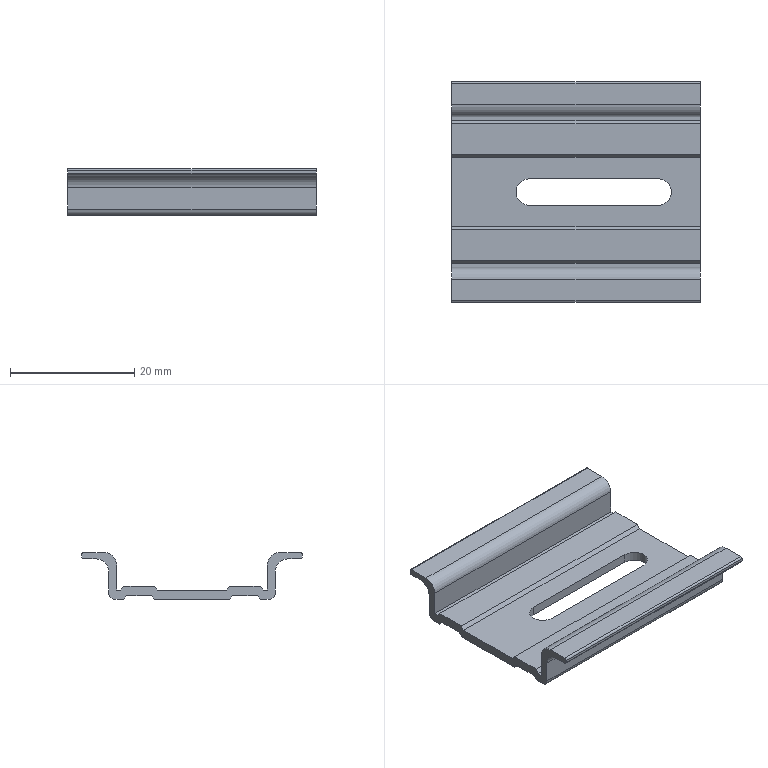Part | NX | features 5003_023_DRAL-5100-100 2 | 1 solid | 44 faces | box 40 x 35.457 x 7.5 mm | volume 2447 mm3 | plane 32 | cylinder 12 | commonest cylinder face diameters 0.6 x4 4 x4 2 x2 4.25 x2
STEP:
#1=CARTESIAN_POINT('',(243.525,-115.4,-99.5));
#2=VERTEX_POINT('',#1);
#3=CARTESIAN_POINT('',(243.525,-115.4,-103.));
#4=VERTEX_POINT('',#3);
#5=CARTESIAN_POINT('',(243.525,-115.4,-99.5));
#6=DIRECTION('',(0.,0.,-1.));
#7=VECTOR('',#6,1000.);
#8=LINE('',#5,#7);
#9=EDGE_CURVE('',#2,#4,#8,.T.);
#10=ORIENTED_EDGE('',*,*,#9,.T.);
#11=CARTESIAN_POINT('',(283.525,-115.4,-103.));
#12=VERTEX_POINT('',#11);
#13=CARTESIAN_POINT('',(283.525,-115.4,-103.));
#14=DIRECTION('',(-1.,0.,0.));
#15=VECTOR('',#14,1000.);
#16=LINE('',#13,#15);
#17=EDGE_CURVE('',#12,#4,#16,.T.);
#18=ORIENTED_EDGE('',*,*,#17,.F.);
#19=CARTESIAN_POINT('',(283.525,-115.4,-99.5));
#20=VERTEX_POINT('',#19);
#21=CARTESIAN_POINT('',(283.525,-115.4,-99.5));
#22=DIRECTION('',(0.,0.,-1.));
#23=VECTOR('',#22,1000.);
#24=LINE('',#21,#23);
#25=EDGE_CURVE('',#20,#12,#24,.T.);
#26=ORIENTED_EDGE('',*,*,#25,.F.);
#27=CARTESIAN_POINT('',(283.525,-115.4,-99.5));
#28=DIRECTION('',(-1.,0.,0.));
#29=VECTOR('',#28,1000.);
#30=LINE('',#27,#29);
#31=EDGE_CURVE('',#20,#2,#30,.T.);
#32=ORIENTED_EDGE('',*,*,#31,.T.);
#33=EDGE_LOOP('',(#10,#18,#26,#32));
#34=FACE_BOUND('',#33,.T.);
#35=CARTESIAN_POINT('',(283.525,-115.4,-99.5));
#36=DIRECTION('',(0.,1.,0.));
#37=DIRECTION('',(-1.,0.,0.));
#38=AXIS2_PLACEMENT_3D('',#35,#36,#37);
#39=PLANE('',#38);
#40=ADVANCED_FACE('',(#34),#39,.F.);
#41=CARTESIAN_POINT('',(243.525,-114.4,-104.));
#42=VERTEX_POINT('',#41);
#43=CARTESIAN_POINT('',(243.525,-114.4,-103.));
#44=DIRECTION('',(1.,0.,0.));
#45=DIRECTION('',(0.,1.,0.));
#46=AXIS2_PLACEMENT_3D('',#43,#44,#45);
#47=CIRCLE('',#46,1.);
#48=EDGE_CURVE('',#4,#42,#47,.T.);
#49=ORIENTED_EDGE('',*,*,#48,.T.);
#50=CARTESIAN_POINT('',(283.525,-114.4,-104.));
#51=VERTEX_POINT('',#50);
#52=CARTESIAN_POINT('',(283.525,-114.4,-104.));
#53=DIRECTION('',(-1.,0.,0.));
#54=VECTOR('',#53,1000.);
#55=LINE('',#52,#54);
#56=EDGE_CURVE('',#51,#42,#55,.T.);
#57=ORIENTED_EDGE('',*,*,#56,.F.);
#58=CARTESIAN_POINT('',(283.525,-114.4,-103.));
#59=DIRECTION('',(1.,0.,0.));
#60=DIRECTION('',(0.,1.,0.));
#61=AXIS2_PLACEMENT_3D('',#58,#59,#60);
#62=CIRCLE('',#61,1.);
#63=EDGE_CURVE('',#12,#51,#62,.T.);
#64=ORIENTED_EDGE('',*,*,#63,.F.);
#65=ORIENTED_EDGE('',*,*,#17,.T.);
#66=EDGE_LOOP('',(#49,#57,#64,#65));
#67=FACE_BOUND('',#66,.T.);
#68=CARTESIAN_POINT('',(283.525,-114.4,-103.));
#69=DIRECTION('',(-1.,0.,0.));
#70=DIRECTION('',(0.,-1.,0.));
#71=AXIS2_PLACEMENT_3D('',#68,#69,#70);
#72=CYLINDRICAL_SURFACE('',#71,1.);
#73=ADVANCED_FACE('',(#67),#72,.T.);
#74=CARTESIAN_POINT('',(243.525,-113.,-104.));
#75=VERTEX_POINT('',#74);
#76=CARTESIAN_POINT('',(243.525,-113.,-104.));
#77=DIRECTION('',(0.,-1.,0.));
#78=VECTOR('',#77,1000.);
#79=LINE('',#76,#78);
#80=EDGE_CURVE('',#75,#42,#79,.T.);
#81=ORIENTED_EDGE('',*,*,#80,.F.);
#82=CARTESIAN_POINT('',(283.525,-113.,-104.));
#83=VERTEX_POINT('',#82);
#84=CARTESIAN_POINT('',(283.525,-113.,-104.));
#85=DIRECTION('',(-1.,0.,0.));
#86=VECTOR('',#85,1000.);
#87=LINE('',#84,#86);
#88=EDGE_CURVE('',#83,#75,#87,.T.);
#89=ORIENTED_EDGE('',*,*,#88,.F.);
#90=CARTESIAN_POINT('',(283.525,-113.,-104.));
#91=DIRECTION('',(0.,-1.,0.));
#92=VECTOR('',#91,1000.);
#93=LINE('',#90,#92);
#94=EDGE_CURVE('',#83,#51,#93,.T.);
#95=ORIENTED_EDGE('',*,*,#94,.T.);
#96=ORIENTED_EDGE('',*,*,#56,.T.);
#97=EDGE_LOOP('',(#81,#89,#95,#96));
#98=FACE_BOUND('',#97,.T.);
#99=CARTESIAN_POINT('',(283.525,-113.,-104.));
#100=DIRECTION('',(0.,0.,-1.));
#101=DIRECTION('',(0.,1.,0.));
#102=AXIS2_PLACEMENT_3D('',#99,#100,#101);
#103=PLANE('',#102);
#104=ADVANCED_FACE('',(#98),#103,.T.);
#105=CARTESIAN_POINT('',(243.525,-112.5,-103.4));
#106=VERTEX_POINT('',#105);
#107=CARTESIAN_POINT('',(243.525,-112.5,-103.4));
#108=DIRECTION('',(0.,-0.6402,-0.7682));
#109=VECTOR('',#108,1000.);
#110=LINE('',#107,#109);
#111=EDGE_CURVE('',#106,#75,#110,.T.);
#112=ORIENTED_EDGE('',*,*,#111,.F.);
#113=CARTESIAN_POINT('',(283.525,-112.5,-103.4));
#114=VERTEX_POINT('',#113);
#115=CARTESIAN_POINT('',(283.525,-112.5,-103.4));
#116=DIRECTION('',(-1.,0.,0.));
#117=VECTOR('',#116,1000.);
#118=LINE('',#115,#117);
#119=EDGE_CURVE('',#114,#106,#118,.T.);
#120=ORIENTED_EDGE('',*,*,#119,.F.);
#121=CARTESIAN_POINT('',(283.525,-112.5,-103.4));
#122=DIRECTION('',(0.,-0.6402,-0.7682));
#123=VECTOR('',#122,1000.);
#124=LINE('',#121,#123);
#125=EDGE_CURVE('',#114,#83,#124,.T.);
#126=ORIENTED_EDGE('',*,*,#125,.T.);
#127=ORIENTED_EDGE('',*,*,#88,.T.);
#128=EDGE_LOOP('',(#112,#120,#126,#127));
#129=FACE_BOUND('',#128,.T.);
#130=CARTESIAN_POINT('',(283.525,-112.5,-103.4));
#131=DIRECTION('',(0.,0.7682,-0.6402));
#132=DIRECTION('',(0.,0.6402,0.7682));
#133=AXIS2_PLACEMENT_3D('',#130,#131,#132);
#134=PLANE('',#133);
#135=ADVANCED_FACE('',(#129),#134,.T.);
#136=CARTESIAN_POINT('',(243.525,-108.5,-103.4));
#137=VERTEX_POINT('',#136);
#138=CARTESIAN_POINT('',(243.525,-108.5,-103.4));
#139=DIRECTION('',(0.,-1.,0.));
#140=VECTOR('',#139,1000.);
#141=LINE('',#138,#140);
#142=EDGE_CURVE('',#137,#106,#141,.T.);
#143=ORIENTED_EDGE('',*,*,#142,.F.);
#144=CARTESIAN_POINT('',(283.525,-108.5,-103.4));
#145=VERTEX_POINT('',#144);
#146=CARTESIAN_POINT('',(283.525,-108.5,-103.4));
#147=DIRECTION('',(-1.,0.,0.));
#148=VECTOR('',#147,1000.);
#149=LINE('',#146,#148);
#150=EDGE_CURVE('',#145,#137,#149,.T.);
#151=ORIENTED_EDGE('',*,*,#150,.F.);
#152=CARTESIAN_POINT('',(283.525,-108.5,-103.4));
#153=DIRECTION('',(0.,-1.,0.));
#154=VECTOR('',#153,1000.);
#155=LINE('',#152,#154);
#156=EDGE_CURVE('',#145,#114,#155,.T.);
#157=ORIENTED_EDGE('',*,*,#156,.T.);
#158=ORIENTED_EDGE('',*,*,#119,.T.);
#159=EDGE_LOOP('',(#143,#151,#157,#158));
#160=FACE_BOUND('',#159,.T.);
#161=CARTESIAN_POINT('',(283.525,-108.5,-103.4));
#162=DIRECTION('',(0.,0.,-1.));
#163=DIRECTION('',(0.,1.,0.));
#164=AXIS2_PLACEMENT_3D('',#161,#162,#163);
#165=PLANE('',#164);
#166=ADVANCED_FACE('',(#160),#165,.T.);
#167=CARTESIAN_POINT('',(243.525,-108.,-104.));
#168=VERTEX_POINT('',#167);
#169=CARTESIAN_POINT('',(243.525,-108.,-104.));
#170=DIRECTION('',(0.,-0.6402,0.7682));
#171=VECTOR('',#170,1000.);
#172=LINE('',#169,#171);
#173=EDGE_CURVE('',#168,#137,#172,.T.);
#174=ORIENTED_EDGE('',*,*,#173,.F.);
#175=CARTESIAN_POINT('',(283.525,-108.,-104.));
#176=VERTEX_POINT('',#175);
#177=CARTESIAN_POINT('',(283.525,-108.,-104.));
#178=DIRECTION('',(-1.,0.,0.));
#179=VECTOR('',#178,1000.);
#180=LINE('',#177,#179);
#181=EDGE_CURVE('',#176,#168,#180,.T.);
#182=ORIENTED_EDGE('',*,*,#181,.F.);
#183=CARTESIAN_POINT('',(283.525,-108.,-104.));
#184=DIRECTION('',(0.,-0.6402,0.7682));
#185=VECTOR('',#184,1000.);
#186=LINE('',#183,#185);
#187=EDGE_CURVE('',#176,#145,#186,.T.);
#188=ORIENTED_EDGE('',*,*,#187,.T.);
#189=ORIENTED_EDGE('',*,*,#150,.T.);
#190=EDGE_LOOP('',(#174,#182,#188,#189));
#191=FACE_BOUND('',#190,.T.);
#192=CARTESIAN_POINT('',(283.525,-108.,-104.));
#193=DIRECTION('',(0.,-0.7682,-0.6402));
#194=DIRECTION('',(0.,0.6402,-0.7682));
#195=AXIS2_PLACEMENT_3D('',#192,#193,#194);
#196=PLANE('',#195);
#197=ADVANCED_FACE('',(#191),#196,.T.);
#198=CARTESIAN_POINT('',(256.005,-104.125,-104.));
#199=VERTEX_POINT('',#198);
#200=CARTESIAN_POINT('',(256.005,-99.875,-104.));
#201=VERTEX_POINT('',#200);
#202=CARTESIAN_POINT('',(256.005,-102.,-104.));
#203=DIRECTION('',(0.,0.,-1.));
#204=DIRECTION('',(0.,1.,0.));
#205=AXIS2_PLACEMENT_3D('',#202,#203,#204);
#206=CIRCLE('',#205,2.125);
#207=EDGE_CURVE('',#199,#201,#206,.T.);
#208=ORIENTED_EDGE('',*,*,#207,.F.);
#209=CARTESIAN_POINT('',(276.755,-104.125,-104.));
#210=VERTEX_POINT('',#209);
#211=CARTESIAN_POINT('',(283.525,-104.125,-104.));
#212=DIRECTION('',(-1.,0.,0.));
#213=VECTOR('',#212,1000.);
#214=LINE('',#211,#213);
#215=EDGE_CURVE('',#210,#199,#214,.T.);
#216=ORIENTED_EDGE('',*,*,#215,.F.);
#217=CARTESIAN_POINT('',(276.755,-99.875,-104.));
#218=VERTEX_POINT('',#217);
#219=CARTESIAN_POINT('',(276.755,-102.,-104.));
#220=DIRECTION('',(0.,0.,-1.));
#221=DIRECTION('',(0.,1.,0.));
#222=AXIS2_PLACEMENT_3D('',#219,#220,#221);
#223=CIRCLE('',#222,2.125);
#224=EDGE_CURVE('',#218,#210,#223,.T.);
#225=ORIENTED_EDGE('',*,*,#224,.F.);
#226=CARTESIAN_POINT('',(283.525,-99.875,-104.));
#227=DIRECTION('',(-1.,0.,0.));
#228=VECTOR('',#227,1000.);
#229=LINE('',#226,#228);
#230=EDGE_CURVE('',#218,#201,#229,.T.);
#231=ORIENTED_EDGE('',*,*,#230,.T.);
#232=EDGE_LOOP('',(#208,#216,#225,#231));
#233=FACE_BOUND('',#232,.T.);
#234=CARTESIAN_POINT('',(243.525,-96.,-104.));
#235=VERTEX_POINT('',#234);
#236=CARTESIAN_POINT('',(243.525,-96.,-104.));
#237=DIRECTION('',(0.,-1.,0.));
#238=VECTOR('',#237,1000.);
#239=LINE('',#236,#238);
#240=EDGE_CURVE('',#235,#168,#239,.T.);
#241=ORIENTED_EDGE('',*,*,#240,.F.);
#242=CARTESIAN_POINT('',(283.525,-96.,-104.));
#243=VERTEX_POINT('',#242);
#244=CARTESIAN_POINT('',(283.525,-96.,-104.));
#245=DIRECTION('',(-1.,0.,0.));
#246=VECTOR('',#245,1000.);
#247=LINE('',#244,#246);
#248=EDGE_CURVE('',#243,#235,#247,.T.);
#249=ORIENTED_EDGE('',*,*,#248,.F.);
#250=CARTESIAN_POINT('',(283.525,-96.,-104.));
#251=DIRECTION('',(0.,-1.,0.));
#252=VECTOR('',#251,1000.);
#253=LINE('',#250,#252);
#254=EDGE_CURVE('',#243,#176,#253,.T.);
#255=ORIENTED_EDGE('',*,*,#254,.T.);
#256=ORIENTED_EDGE('',*,*,#181,.T.);
#257=EDGE_LOOP('',(#241,#249,#255,#256));
#258=FACE_BOUND('',#257,.T.);
#259=CARTESIAN_POINT('',(283.525,-96.,-104.));
#260=DIRECTION('',(0.,0.,-1.));
#261=DIRECTION('',(0.,1.,0.));
#262=AXIS2_PLACEMENT_3D('',#259,#260,#261);
#263=PLANE('',#262);
#264=ADVANCED_FACE('',(#233,#258),#263,.T.);
#265=CARTESIAN_POINT('',(243.525,-95.5,-103.4));
#266=VERTEX_POINT('',#265);
#267=CARTESIAN_POINT('',(243.525,-96.,-104.));
#268=DIRECTION('',(0.,0.6402,0.7682));
#269=VECTOR('',#268,1000.);
#270=LINE('',#267,#269);
#271=EDGE_CURVE('',#235,#266,#270,.T.);
#272=ORIENTED_EDGE('',*,*,#271,.T.);
#273=CARTESIAN_POINT('',(283.525,-95.5,-103.4));
#274=VERTEX_POINT('',#273);
#275=CARTESIAN_POINT('',(283.525,-95.5,-103.4));
#276=DIRECTION('',(-1.,0.,0.));
#277=VECTOR('',#276,1000.);
#278=LINE('',#275,#277);
#279=EDGE_CURVE('',#274,#266,#278,.T.);
#280=ORIENTED_EDGE('',*,*,#279,.F.);
#281=CARTESIAN_POINT('',(283.525,-96.,-104.));
#282=DIRECTION('',(0.,0.6402,0.7682));
#283=VECTOR('',#282,1000.);
#284=LINE('',#281,#283);
#285=EDGE_CURVE('',#243,#274,#284,.T.);
#286=ORIENTED_EDGE('',*,*,#285,.F.);
#287=ORIENTED_EDGE('',*,*,#248,.T.);
#288=EDGE_LOOP('',(#272,#280,#286,#287));
#289=FACE_BOUND('',#288,.T.);
#290=CARTESIAN_POINT('',(283.525,-96.,-104.));
#291=DIRECTION('',(0.,-0.7682,0.6402));
#292=DIRECTION('',(0.,-0.6402,-0.7682));
#293=AXIS2_PLACEMENT_3D('',#290,#291,#292);
#294=PLANE('',#293);
#295=ADVANCED_FACE('',(#289),#294,.F.);
#296=CARTESIAN_POINT('',(243.525,-91.5,-103.4));
#297=VERTEX_POINT('',#296);
#298=CARTESIAN_POINT('',(243.525,-95.5,-103.4));
#299=DIRECTION('',(0.,1.,0.));
#300=VECTOR('',#299,1000.);
#301=LINE('',#298,#300);
#302=EDGE_CURVE('',#266,#297,#301,.T.);
#303=ORIENTED_EDGE('',*,*,#302,.T.);
#304=CARTESIAN_POINT('',(283.525,-91.5,-103.4));
#305=VERTEX_POINT('',#304);
#306=CARTESIAN_POINT('',(283.525,-91.5,-103.4));
#307=DIRECTION('',(-1.,0.,0.));
#308=VECTOR('',#307,1000.);
#309=LINE('',#306,#308);
#310=EDGE_CURVE('',#305,#297,#309,.T.);
#311=ORIENTED_EDGE('',*,*,#310,.F.);
#312=CARTESIAN_POINT('',(283.525,-95.5,-103.4));
#313=DIRECTION('',(0.,1.,0.));
#314=VECTOR('',#313,1000.);
#315=LINE('',#312,#314);
#316=EDGE_CURVE('',#274,#305,#315,.T.);
#317=ORIENTED_EDGE('',*,*,#316,.F.);
#318=ORIENTED_EDGE('',*,*,#279,.T.);
#319=EDGE_LOOP('',(#303,#311,#317,#318));
#320=FACE_BOUND('',#319,.T.);
#321=CARTESIAN_POINT('',(283.525,-95.5,-103.4));
#322=DIRECTION('',(0.,0.,1.));
#323=DIRECTION('',(0.,-1.,0.));
#324=AXIS2_PLACEMENT_3D('',#321,#322,#323);
#325=PLANE('',#324);
#326=ADVANCED_FACE('',(#320),#325,.F.);
#327=CARTESIAN_POINT('',(243.525,-91.,-104.));
#328=VERTEX_POINT('',#327);
#329=CARTESIAN_POINT('',(243.525,-91.5,-103.4));
#330=DIRECTION('',(0.,0.6402,-0.7682));
#331=VECTOR('',#330,1000.);
#332=LINE('',#329,#331);
#333=EDGE_CURVE('',#297,#328,#332,.T.);
#334=ORIENTED_EDGE('',*,*,#333,.T.);
#335=CARTESIAN_POINT('',(283.525,-91.,-104.));
#336=VERTEX_POINT('',#335);
#337=CARTESIAN_POINT('',(283.525,-91.,-104.));
#338=DIRECTION('',(-1.,0.,0.));
#339=VECTOR('',#338,1000.);
#340=LINE('',#337,#339);
#341=EDGE_CURVE('',#336,#328,#340,.T.);
#342=ORIENTED_EDGE('',*,*,#341,.F.);
#343=CARTESIAN_POINT('',(283.525,-91.5,-103.4));
#344=DIRECTION('',(0.,0.6402,-0.7682));
#345=VECTOR('',#344,1000.);
#346=LINE('',#343,#345);
#347=EDGE_CURVE('',#305,#336,#346,.T.);
#348=ORIENTED_EDGE('',*,*,#347,.F.);
#349=ORIENTED_EDGE('',*,*,#310,.T.);
#350=EDGE_LOOP('',(#334,#342,#348,#349));
#351=FACE_BOUND('',#350,.T.);
#352=CARTESIAN_POINT('',(283.525,-91.5,-103.4));
#353=DIRECTION('',(0.,0.7682,0.6402));
#354=DIRECTION('',(0.,-0.6402,0.7682));
#355=AXIS2_PLACEMENT_3D('',#352,#353,#354);
#356=PLANE('',#355);
#357=ADVANCED_FACE('',(#351),#356,.F.);
#358=CARTESIAN_POINT('',(243.525,-89.6,-104.));
#359=VERTEX_POINT('',#358);
#360=CARTESIAN_POINT('',(243.525,-91.,-104.));
#361=DIRECTION('',(0.,1.,0.));
#362=VECTOR('',#361,1000.);
#363=LINE('',#360,#362);
#364=EDGE_CURVE('',#328,#359,#363,.T.);
#365=ORIENTED_EDGE('',*,*,#364,.T.);
#366=CARTESIAN_POINT('',(283.525,-89.6,-104.));
#367=VERTEX_POINT('',#366);
#368=CARTESIAN_POINT('',(283.525,-89.6,-104.));
#369=DIRECTION('',(-1.,0.,0.));
#370=VECTOR('',#369,1000.);
#371=LINE('',#368,#370);
#372=EDGE_CURVE('',#367,#359,#371,.T.);
#373=ORIENTED_EDGE('',*,*,#372,.F.);
#374=CARTESIAN_POINT('',(283.525,-91.,-104.));
#375=DIRECTION('',(0.,1.,0.));
#376=VECTOR('',#375,1000.);
#377=LINE('',#374,#376);
#378=EDGE_CURVE('',#336,#367,#377,.T.);
#379=ORIENTED_EDGE('',*,*,#378,.F.);
#380=ORIENTED_EDGE('',*,*,#341,.T.);
#381=EDGE_LOOP('',(#365,#373,#379,#380));
#382=FACE_BOUND('',#381,.T.);
#383=CARTESIAN_POINT('',(283.525,-91.,-104.));
#384=DIRECTION('',(0.,0.,1.));
#385=DIRECTION('',(0.,-1.,0.));
#386=AXIS2_PLACEMENT_3D('',#383,#384,#385);
#387=PLANE('',#386);
#388=ADVANCED_FACE('',(#382),#387,.F.);
#389=CARTESIAN_POINT('',(243.525,-88.6,-103.));
#390=VERTEX_POINT('',#389);
#391=CARTESIAN_POINT('',(243.525,-89.6,-103.));
#392=DIRECTION('',(-1.,0.,0.));
#393=DIRECTION('',(0.,-1.,0.));
#394=AXIS2_PLACEMENT_3D('',#391,#392,#393);
#395=CIRCLE('',#394,1.);
#396=EDGE_CURVE('',#390,#359,#395,.T.);
#397=ORIENTED_EDGE('',*,*,#396,.F.);
#398=CARTESIAN_POINT('',(283.525,-88.6,-103.));
#399=VERTEX_POINT('',#398);
#400=CARTESIAN_POINT('',(283.525,-88.6,-103.));
#401=DIRECTION('',(-1.,0.,0.));
#402=VECTOR('',#401,1000.);
#403=LINE('',#400,#402);
#404=EDGE_CURVE('',#399,#390,#403,.T.);
#405=ORIENTED_EDGE('',*,*,#404,.F.);
#406=CARTESIAN_POINT('',(283.525,-89.6,-103.));
#407=DIRECTION('',(-1.,0.,0.));
#408=DIRECTION('',(0.,-1.,0.));
#409=AXIS2_PLACEMENT_3D('',#406,#407,#408);
#410=CIRCLE('',#409,1.);
#411=EDGE_CURVE('',#399,#367,#410,.T.);
#412=ORIENTED_EDGE('',*,*,#411,.T.);
#413=ORIENTED_EDGE('',*,*,#372,.T.);
#414=EDGE_LOOP('',(#397,#405,#412,#413));
#415=FACE_BOUND('',#414,.T.);
#416=CARTESIAN_POINT('',(283.525,-89.6,-103.));
#417=DIRECTION('',(-1.,0.,0.));
#418=DIRECTION('',(0.,-1.,0.));
#419=AXIS2_PLACEMENT_3D('',#416,#417,#418);
#420=CYLINDRICAL_SURFACE('',#419,1.);
#421=ADVANCED_FACE('',(#415),#420,.T.);
#422=CARTESIAN_POINT('',(243.525,-88.6,-99.5));
#423=VERTEX_POINT('',#422);
#424=CARTESIAN_POINT('',(243.525,-88.6,-99.5));
#425=DIRECTION('',(0.,0.,-1.));
#426=VECTOR('',#425,1000.);
#427=LINE('',#424,#426);
#428=EDGE_CURVE('',#423,#390,#427,.T.);
#429=ORIENTED_EDGE('',*,*,#428,.F.);
#430=CARTESIAN_POINT('',(283.525,-88.6,-99.5));
#431=VERTEX_POINT('',#430);
#432=CARTESIAN_POINT('',(283.525,-88.6,-99.5));
#433=DIRECTION('',(-1.,0.,0.));
#434=VECTOR('',#433,1000.);
#435=LINE('',#432,#434);
#436=EDGE_CURVE('',#431,#423,#435,.T.);
#437=ORIENTED_EDGE('',*,*,#436,.F.);
#438=CARTESIAN_POINT('',(283.525,-88.6,-99.5));
#439=DIRECTION('',(0.,0.,-1.));
#440=VECTOR('',#439,1000.);
#441=LINE('',#438,#440);
#442=EDGE_CURVE('',#431,#399,#441,.T.);
#443=ORIENTED_EDGE('',*,*,#442,.T.);
#444=ORIENTED_EDGE('',*,*,#404,.T.);
#445=EDGE_LOOP('',(#429,#437,#443,#444));
#446=FACE_BOUND('',#445,.T.);
#447=CARTESIAN_POINT('',(283.525,-88.6,-99.5));
#448=DIRECTION('',(0.,1.,0.));
#449=DIRECTION('',(-1.,0.,0.));
#450=AXIS2_PLACEMENT_3D('',#447,#448,#449);
#451=PLANE('',#450);
#452=ADVANCED_FACE('',(#446),#451,.T.);
#453=CARTESIAN_POINT('',(243.525,-86.6,-97.5));
#454=VERTEX_POINT('',#453);
#455=CARTESIAN_POINT('',(243.525,-86.6,-99.5));
#456=DIRECTION('',(-1.,0.,0.));
#457=DIRECTION('',(0.,-1.,0.));
#458=AXIS2_PLACEMENT_3D('',#455,#456,#457);
#459=CIRCLE('',#458,2.);
#460=EDGE_CURVE('',#423,#454,#459,.T.);
#461=ORIENTED_EDGE('',*,*,#460,.T.);
#462=CARTESIAN_POINT('',(283.525,-86.6,-97.5));
#463=VERTEX_POINT('',#462);
#464=CARTESIAN_POINT('',(283.525,-86.6,-97.5));
#465=DIRECTION('',(-1.,0.,0.));
#466=VECTOR('',#465,1000.);
#467=LINE('',#464,#466);
#468=EDGE_CURVE('',#463,#454,#467,.T.);
#469=ORIENTED_EDGE('',*,*,#468,.F.);
#470=CARTESIAN_POINT('',(283.525,-86.6,-99.5));
#471=DIRECTION('',(-1.,0.,0.));
#472=DIRECTION('',(0.,-1.,0.));
#473=AXIS2_PLACEMENT_3D('',#470,#471,#472);
#474=CIRCLE('',#473,2.);
#475=EDGE_CURVE('',#431,#463,#474,.T.);
#476=ORIENTED_EDGE('',*,*,#475,.F.);
#477=ORIENTED_EDGE('',*,*,#436,.T.);
#478=EDGE_LOOP('',(#461,#469,#476,#477));
#479=FACE_BOUND('',#478,.T.);
#480=CARTESIAN_POINT('',(283.525,-86.6,-99.5));
#481=DIRECTION('',(-1.,0.,0.));
#482=DIRECTION('',(0.,-1.,0.));
#483=AXIS2_PLACEMENT_3D('',#480,#481,#482);
#484=CYLINDRICAL_SURFACE('',#483,2.);
#485=ADVANCED_FACE('',(#479),#484,.F.);
#486=CARTESIAN_POINT('',(243.525,-84.572,-97.5));
#487=VERTEX_POINT('',#486);
#488=CARTESIAN_POINT('',(243.525,-86.6,-97.5));
#489=DIRECTION('',(0.,1.,0.));
#490=VECTOR('',#489,1000.);
#491=LINE('',#488,#490);
#492=EDGE_CURVE('',#454,#487,#491,.T.);
#493=ORIENTED_EDGE('',*,*,#492,.T.);
#494=CARTESIAN_POINT('',(283.525,-84.572,-97.5));
#495=VERTEX_POINT('',#494);
#496=CARTESIAN_POINT('',(283.525,-84.572,-97.5));
#497=DIRECTION('',(-1.,0.,0.));
#498=VECTOR('',#497,1000.);
#499=LINE('',#496,#498);
#500=EDGE_CURVE('',#495,#487,#499,.T.);
#501=ORIENTED_EDGE('',*,*,#500,.F.);
#502=CARTESIAN_POINT('',(283.525,-86.6,-97.5));
#503=DIRECTION('',(0.,1.,0.));
#504=VECTOR('',#503,1000.);
#505=LINE('',#502,#504);
#506=EDGE_CURVE('',#463,#495,#505,.T.);
#507=ORIENTED_EDGE('',*,*,#506,.F.);
#508=ORIENTED_EDGE('',*,*,#468,.T.);
#509=EDGE_LOOP('',(#493,#501,#507,#508));
#510=FACE_BOUND('',#509,.T.);
#511=CARTESIAN_POINT('',(283.525,-86.6,-97.5));
#512=DIRECTION('',(0.,0.,1.));
#513=DIRECTION('',(0.,-1.,0.));
#514=AXIS2_PLACEMENT_3D('',#511,#512,#513);
#515=PLANE('',#514);
#516=ADVANCED_FACE('',(#510),#515,.F.);
#517=CARTESIAN_POINT('',(243.525,-84.272,-97.2));
#518=VERTEX_POINT('',#517);
#519=CARTESIAN_POINT('',(243.525,-84.572,-97.2));
#520=DIRECTION('',(-1.,0.,0.));
#521=DIRECTION('',(0.,-1.,0.));
#522=AXIS2_PLACEMENT_3D('',#519,#520,#521);
#523=CIRCLE('',#522,0.3);
#524=EDGE_CURVE('',#518,#487,#523,.T.);
#525=ORIENTED_EDGE('',*,*,#524,.F.);
#526=CARTESIAN_POINT('',(283.525,-84.272,-97.2));
#527=VERTEX_POINT('',#526);
#528=CARTESIAN_POINT('',(283.525,-84.272,-97.2));
#529=DIRECTION('',(-1.,0.,0.));
#530=VECTOR('',#529,1000.);
#531=LINE('',#528,#530);
#532=EDGE_CURVE('',#527,#518,#531,.T.);
#533=ORIENTED_EDGE('',*,*,#532,.F.);
#534=CARTESIAN_POINT('',(283.525,-84.572,-97.2));
#535=DIRECTION('',(-1.,0.,0.));
#536=DIRECTION('',(0.,-1.,0.));
#537=AXIS2_PLACEMENT_3D('',#534,#535,#536);
#538=CIRCLE('',#537,0.3);
#539=EDGE_CURVE('',#527,#495,#538,.T.);
#540=ORIENTED_EDGE('',*,*,#539,.T.);
#541=ORIENTED_EDGE('',*,*,#500,.T.);
#542=EDGE_LOOP('',(#525,#533,#540,#541));
#543=FACE_BOUND('',#542,.T.);
#544=CARTESIAN_POINT('',(283.525,-84.572,-97.2));
#545=DIRECTION('',(-1.,0.,0.));
#546=DIRECTION('',(0.,-1.,0.));
#547=AXIS2_PLACEMENT_3D('',#544,#545,#546);
#548=CYLINDRICAL_SURFACE('',#547,0.3);
#549=ADVANCED_FACE('',(#543),#548,.T.);
#550=CARTESIAN_POINT('',(243.525,-84.272,-96.8));
#551=VERTEX_POINT('',#550);
#552=CARTESIAN_POINT('',(243.525,-84.272,-97.2));
#553=DIRECTION('',(0.,0.,1.));
#554=VECTOR('',#553,1000.);
#555=LINE('',#552,#554);
#556=EDGE_CURVE('',#518,#551,#555,.T.);
#557=ORIENTED_EDGE('',*,*,#556,.T.);
#558=CARTESIAN_POINT('',(283.525,-84.272,-96.8));
#559=VERTEX_POINT('',#558);
#560=CARTESIAN_POINT('',(283.525,-84.272,-96.8));
#561=DIRECTION('',(-1.,0.,0.));
#562=VECTOR('',#561,1000.);
#563=LINE('',#560,#562);
#564=EDGE_CURVE('',#559,#551,#563,.T.);
#565=ORIENTED_EDGE('',*,*,#564,.F.);
#566=CARTESIAN_POINT('',(283.525,-84.272,-97.2));
#567=DIRECTION('',(0.,0.,1.));
#568=VECTOR('',#567,1000.);
#569=LINE('',#566,#568);
#570=EDGE_CURVE('',#527,#559,#569,.T.);
#571=ORIENTED_EDGE('',*,*,#570,.F.);
#572=ORIENTED_EDGE('',*,*,#532,.T.);
#573=EDGE_LOOP('',(#557,#565,#571,#572));
#574=FACE_BOUND('',#573,.T.);
#575=CARTESIAN_POINT('',(283.525,-84.272,-97.2));
#576=DIRECTION('',(0.,-1.,0.));
#577=DIRECTION('',(1.,0.,0.));
#578=AXIS2_PLACEMENT_3D('',#575,#576,#577);
#579=PLANE('',#578);
#580=ADVANCED_FACE('',(#574),#579,.F.);
#581=CARTESIAN_POINT('',(243.525,-84.572,-96.5));
#582=VERTEX_POINT('',#581);
#583=CARTESIAN_POINT('',(243.525,-84.572,-96.8));
#584=DIRECTION('',(-1.,0.,0.));
#585=DIRECTION('',(0.,-1.,0.));
#586=AXIS2_PLACEMENT_3D('',#583,#584,#585);
#587=CIRCLE('',#586,0.3);
#588=EDGE_CURVE('',#582,#551,#587,.T.);
#589=ORIENTED_EDGE('',*,*,#588,.F.);
#590=CARTESIAN_POINT('',(283.525,-84.572,-96.5));
#591=VERTEX_POINT('',#590);
#592=CARTESIAN_POINT('',(283.525,-84.572,-96.5));
#593=DIRECTION('',(-1.,0.,0.));
#594=VECTOR('',#593,1000.);
#595=LINE('',#592,#594);
#596=EDGE_CURVE('',#591,#582,#595,.T.);
#597=ORIENTED_EDGE('',*,*,#596,.F.);
#598=CARTESIAN_POINT('',(283.525,-84.572,-96.8));
#599=DIRECTION('',(-1.,0.,0.));
#600=DIRECTION('',(0.,-1.,0.));
#601=AXIS2_PLACEMENT_3D('',#598,#599,#600);
#602=CIRCLE('',#601,0.3);
#603=EDGE_CURVE('',#591,#559,#602,.T.);
#604=ORIENTED_EDGE('',*,*,#603,.T.);
#605=ORIENTED_EDGE('',*,*,#564,.T.);
#606=EDGE_LOOP('',(#589,#597,#604,#605));
#607=FACE_BOUND('',#606,.T.);
#608=CARTESIAN_POINT('',(283.525,-84.572,-96.8));
#609=DIRECTION('',(-1.,0.,0.));
#610=DIRECTION('',(0.,-1.,0.));
#611=AXIS2_PLACEMENT_3D('',#608,#609,#610);
#612=CYLINDRICAL_SURFACE('',#611,0.3);
#613=ADVANCED_FACE('',(#607),#612,.T.);
#614=CARTESIAN_POINT('',(243.525,-87.9,-96.5));
#615=VERTEX_POINT('',#614);
#616=CARTESIAN_POINT('',(243.525,-84.572,-96.5));
#617=DIRECTION('',(0.,-1.,0.));
#618=VECTOR('',#617,1000.);
#619=LINE('',#616,#618);
#620=EDGE_CURVE('',#582,#615,#619,.T.);
#621=ORIENTED_EDGE('',*,*,#620,.T.);
#622=CARTESIAN_POINT('',(283.525,-87.9,-96.5));
#623=VERTEX_POINT('',#622);
#624=CARTESIAN_POINT('',(283.525,-87.9,-96.5));
#625=DIRECTION('',(-1.,0.,0.));
#626=VECTOR('',#625,1000.);
#627=LINE('',#624,#626);
#628=EDGE_CURVE('',#623,#615,#627,.T.);
#629=ORIENTED_EDGE('',*,*,#628,.F.);
#630=CARTESIAN_POINT('',(283.525,-84.572,-96.5));
#631=DIRECTION('',(0.,-1.,0.));
#632=VECTOR('',#631,1000.);
#633=LINE('',#630,#632);
#634=EDGE_CURVE('',#591,#623,#633,.T.);
#635=ORIENTED_EDGE('',*,*,#634,.F.);
#636=ORIENTED_EDGE('',*,*,#596,.T.);
#637=EDGE_LOOP('',(#621,#629,#635,#636));
#638=FACE_BOUND('',#637,.T.);
#639=CARTESIAN_POINT('',(283.525,-84.572,-96.5));
#640=DIRECTION('',(0.,0.,-1.));
#641=DIRECTION('',(0.,1.,0.));
#642=AXIS2_PLACEMENT_3D('',#639,#640,#641);
#643=PLANE('',#642);
#644=ADVANCED_FACE('',(#638),#643,.F.);
#645=CARTESIAN_POINT('',(243.525,-89.9,-98.5));
#646=VERTEX_POINT('',#645);
#647=CARTESIAN_POINT('',(243.525,-87.9,-98.5));
#648=DIRECTION('',(-1.,0.,0.));
#649=DIRECTION('',(0.,-1.,0.));
#650=AXIS2_PLACEMENT_3D('',#647,#648,#649);
#651=CIRCLE('',#650,2.);
#652=EDGE_CURVE('',#646,#615,#651,.T.);
#653=ORIENTED_EDGE('',*,*,#652,.F.);
#654=CARTESIAN_POINT('',(283.525,-89.9,-98.5));
#655=VERTEX_POINT('',#654);
#656=CARTESIAN_POINT('',(283.525,-89.9,-98.5));
#657=DIRECTION('',(-1.,0.,0.));
#658=VECTOR('',#657,1000.);
#659=LINE('',#656,#658);
#660=EDGE_CURVE('',#655,#646,#659,.T.);
#661=ORIENTED_EDGE('',*,*,#660,.F.);
#662=CARTESIAN_POINT('',(283.525,-87.9,-98.5));
#663=DIRECTION('',(-1.,0.,0.));
#664=DIRECTION('',(0.,-1.,0.));
#665=AXIS2_PLACEMENT_3D('',#662,#663,#664);
#666=CIRCLE('',#665,2.);
#667=EDGE_CURVE('',#655,#623,#666,.T.);
#668=ORIENTED_EDGE('',*,*,#667,.T.);
#669=ORIENTED_EDGE('',*,*,#628,.T.);
#670=EDGE_LOOP('',(#653,#661,#668,#669));
#671=FACE_BOUND('',#670,.T.);
#672=CARTESIAN_POINT('',(283.525,-87.9,-98.5));
#673=DIRECTION('',(-1.,0.,0.));
#674=DIRECTION('',(0.,-1.,0.));
#675=AXIS2_PLACEMENT_3D('',#672,#673,#674);
#676=CYLINDRICAL_SURFACE('',#675,2.);
#677=ADVANCED_FACE('',(#671),#676,.T.);
#678=CARTESIAN_POINT('',(243.525,-89.9,-102.5));
#679=VERTEX_POINT('',#678);
#680=CARTESIAN_POINT('',(243.525,-89.9,-98.5));
#681=DIRECTION('',(0.,0.,-1.));
#682=VECTOR('',#681,1000.);
#683=LINE('',#680,#682);
#684=EDGE_CURVE('',#646,#679,#683,.T.);
#685=ORIENTED_EDGE('',*,*,#684,.T.);
#686=CARTESIAN_POINT('',(283.525,-89.9,-102.5));
#687=VERTEX_POINT('',#686);
#688=CARTESIAN_POINT('',(283.525,-89.9,-102.5));
#689=DIRECTION('',(-1.,0.,0.));
#690=VECTOR('',#689,1000.);
#691=LINE('',#688,#690);
#692=EDGE_CURVE('',#687,#679,#691,.T.);
#693=ORIENTED_EDGE('',*,*,#692,.F.);
#694=CARTESIAN_POINT('',(283.525,-89.9,-98.5));
#695=DIRECTION('',(0.,0.,-1.));
#696=VECTOR('',#695,1000.);
#697=LINE('',#694,#696);
#698=EDGE_CURVE('',#655,#687,#697,.T.);
#699=ORIENTED_EDGE('',*,*,#698,.F.);
#700=ORIENTED_EDGE('',*,*,#660,.T.);
#701=EDGE_LOOP('',(#685,#693,#699,#700));
#702=FACE_BOUND('',#701,.T.);
#703=CARTESIAN_POINT('',(283.525,-89.9,-98.5));
#704=DIRECTION('',(0.,1.,0.));
#705=DIRECTION('',(0.,0.,1.));
#706=AXIS2_PLACEMENT_3D('',#703,#704,#705);
#707=PLANE('',#706);
#708=ADVANCED_FACE('',(#702),#707,.F.);
#709=CARTESIAN_POINT('',(243.525,-90.558,-102.5));
#710=VERTEX_POINT('',#709);
#711=CARTESIAN_POINT('',(243.525,-89.9,-102.5));
#712=DIRECTION('',(0.,-1.,0.));
#713=VECTOR('',#712,1000.);
#714=LINE('',#711,#713);
#715=EDGE_CURVE('',#679,#710,#714,.T.);
#716=ORIENTED_EDGE('',*,*,#715,.T.);
#717=CARTESIAN_POINT('',(283.525,-90.558,-102.5));
#718=VERTEX_POINT('',#717);
#719=CARTESIAN_POINT('',(283.525,-90.558,-102.5));
#720=DIRECTION('',(-1.,0.,0.));
#721=VECTOR('',#720,1000.);
#722=LINE('',#719,#721);
#723=EDGE_CURVE('',#718,#710,#722,.T.);
#724=ORIENTED_EDGE('',*,*,#723,.F.);
#725=CARTESIAN_POINT('',(283.525,-89.9,-102.5));
#726=DIRECTION('',(0.,-1.,0.));
#727=VECTOR('',#726,1000.);
#728=LINE('',#725,#727);
#729=EDGE_CURVE('',#687,#718,#728,.T.);
#730=ORIENTED_EDGE('',*,*,#729,.F.);
#731=ORIENTED_EDGE('',*,*,#692,.T.);
#732=EDGE_LOOP('',(#716,#724,#730,#731));
#733=FACE_BOUND('',#732,.T.);
#734=CARTESIAN_POINT('',(283.525,-89.9,-102.5));
#735=DIRECTION('',(0.,0.,-1.));
#736=DIRECTION('',(0.,1.,0.));
#737=AXIS2_PLACEMENT_3D('',#734,#735,#736);
#738=PLANE('',#737);
#739=ADVANCED_FACE('',(#733),#738,.F.);
#740=CARTESIAN_POINT('',(243.525,-91.058,-101.9));
#741=VERTEX_POINT('',#740);
#742=CARTESIAN_POINT('',(243.525,-90.558,-102.5));
#743=DIRECTION('',(0.,-0.6402,0.7682));
#744=VECTOR('',#743,1000.);
#745=LINE('',#742,#744);
#746=EDGE_CURVE('',#710,#741,#745,.T.);
#747=ORIENTED_EDGE('',*,*,#746,.T.);
#748=CARTESIAN_POINT('',(283.525,-91.058,-101.9));
#749=VERTEX_POINT('',#748);
#750=CARTESIAN_POINT('',(283.525,-91.058,-101.9));
#751=DIRECTION('',(-1.,0.,0.));
#752=VECTOR('',#751,1000.);
#753=LINE('',#750,#752);
#754=EDGE_CURVE('',#749,#741,#753,.T.);
#755=ORIENTED_EDGE('',*,*,#754,.F.);
#756=CARTESIAN_POINT('',(283.525,-90.558,-102.5));
#757=DIRECTION('',(0.,-0.6402,0.7682));
#758=VECTOR('',#757,1000.);
#759=LINE('',#756,#758);
#760=EDGE_CURVE('',#718,#749,#759,.T.);
#761=ORIENTED_EDGE('',*,*,#760,.F.);
#762=ORIENTED_EDGE('',*,*,#723,.T.);
#763=EDGE_LOOP('',(#747,#755,#761,#762));
#764=FACE_BOUND('',#763,.T.);
#765=CARTESIAN_POINT('',(283.525,-90.558,-102.5));
#766=DIRECTION('',(0.,-0.7682,-0.6402));
#767=DIRECTION('',(0.,0.6402,-0.7682));
#768=AXIS2_PLACEMENT_3D('',#765,#766,#767);
#769=PLANE('',#768);
#770=ADVANCED_FACE('',(#764),#769,.F.);
#771=CARTESIAN_POINT('',(243.525,-95.942,-101.9));
#772=VERTEX_POINT('',#771);
#773=CARTESIAN_POINT('',(243.525,-91.058,-101.9));
#774=DIRECTION('',(0.,-1.,0.));
#775=VECTOR('',#774,1000.);
#776=LINE('',#773,#775);
#777=EDGE_CURVE('',#741,#772,#776,.T.);
#778=ORIENTED_EDGE('',*,*,#777,.T.);
#779=CARTESIAN_POINT('',(283.525,-95.942,-101.9));
#780=VERTEX_POINT('',#779);
#781=CARTESIAN_POINT('',(283.525,-95.942,-101.9));
#782=DIRECTION('',(-1.,0.,0.));
#783=VECTOR('',#782,1000.);
#784=LINE('',#781,#783);
#785=EDGE_CURVE('',#780,#772,#784,.T.);
#786=ORIENTED_EDGE('',*,*,#785,.F.);
#787=CARTESIAN_POINT('',(283.525,-91.058,-101.9));
#788=DIRECTION('',(0.,-1.,0.));
#789=VECTOR('',#788,1000.);
#790=LINE('',#787,#789);
#791=EDGE_CURVE('',#749,#780,#790,.T.);
#792=ORIENTED_EDGE('',*,*,#791,.F.);
#793=ORIENTED_EDGE('',*,*,#754,.T.);
#794=EDGE_LOOP('',(#778,#786,#792,#793));
#795=FACE_BOUND('',#794,.T.);
#796=CARTESIAN_POINT('',(283.525,-91.058,-101.9));
#797=DIRECTION('',(0.,0.,-1.));
#798=DIRECTION('',(0.,1.,0.));
#799=AXIS2_PLACEMENT_3D('',#796,#797,#798);
#800=PLANE('',#799);
#801=ADVANCED_FACE('',(#795),#800,.F.);
#802=CARTESIAN_POINT('',(243.525,-96.442,-102.5));
#803=VERTEX_POINT('',#802);
#804=CARTESIAN_POINT('',(243.525,-95.942,-101.9));
#805=DIRECTION('',(0.,-0.6402,-0.7682));
#806=VECTOR('',#805,1000.);
#807=LINE('',#804,#806);
#808=EDGE_CURVE('',#772,#803,#807,.T.);
#809=ORIENTED_EDGE('',*,*,#808,.T.);
#810=CARTESIAN_POINT('',(283.525,-96.442,-102.5));
#811=VERTEX_POINT('',#810);
#812=CARTESIAN_POINT('',(283.525,-96.442,-102.5));
#813=DIRECTION('',(-1.,0.,0.));
#814=VECTOR('',#813,1000.);
#815=LINE('',#812,#814);
#816=EDGE_CURVE('',#811,#803,#815,.T.);
#817=ORIENTED_EDGE('',*,*,#816,.F.);
#818=CARTESIAN_POINT('',(283.525,-95.942,-101.9));
#819=DIRECTION('',(0.,-0.6402,-0.7682));
#820=VECTOR('',#819,1000.);
#821=LINE('',#818,#820);
#822=EDGE_CURVE('',#780,#811,#821,.T.);
#823=ORIENTED_EDGE('',*,*,#822,.F.);
#824=ORIENTED_EDGE('',*,*,#785,.T.);
#825=EDGE_LOOP('',(#809,#817,#823,#824));
#826=FACE_BOUND('',#825,.T.);
#827=CARTESIAN_POINT('',(283.525,-95.942,-101.9));
#828=DIRECTION('',(0.,0.7682,-0.6402));
#829=DIRECTION('',(0.,0.6402,0.7682));
#830=AXIS2_PLACEMENT_3D('',#827,#828,#829);
#831=PLANE('',#830);
#832=ADVANCED_FACE('',(#826),#831,.F.);
#833=CARTESIAN_POINT('',(256.005,-99.875,-102.5));
#834=VERTEX_POINT('',#833);
#835=CARTESIAN_POINT('',(256.005,-104.125,-102.5));
#836=VERTEX_POINT('',#835);
#837=CARTESIAN_POINT('',(256.005,-102.,-102.5));
#838=DIRECTION('',(0.,0.,1.));
#839=DIRECTION('',(0.,-1.,0.));
#840=AXIS2_PLACEMENT_3D('',#837,#838,#839);
#841=CIRCLE('',#840,2.125);
#842=EDGE_CURVE('',#834,#836,#841,.T.);
#843=ORIENTED_EDGE('',*,*,#842,.F.);
#844=CARTESIAN_POINT('',(276.755,-99.875,-102.5));
#845=VERTEX_POINT('',#844);
#846=CARTESIAN_POINT('',(256.005,-99.875,-102.5));
#847=DIRECTION('',(1.,0.,0.));
#848=VECTOR('',#847,1000.);
#849=LINE('',#846,#848);
#850=EDGE_CURVE('',#834,#845,#849,.T.);
#851=ORIENTED_EDGE('',*,*,#850,.T.);
#852=CARTESIAN_POINT('',(276.755,-104.125,-102.5));
#853=VERTEX_POINT('',#852);
#854=CARTESIAN_POINT('',(276.755,-102.,-102.5));
#855=DIRECTION('',(0.,0.,1.));
#856=DIRECTION('',(0.,-1.,0.));
#857=AXIS2_PLACEMENT_3D('',#854,#855,#856);
#858=CIRCLE('',#857,2.125);
#859=EDGE_CURVE('',#853,#845,#858,.T.);
#860=ORIENTED_EDGE('',*,*,#859,.F.);
#861=CARTESIAN_POINT('',(256.005,-104.125,-102.5));
#862=DIRECTION('',(1.,0.,0.));
#863=VECTOR('',#862,1000.);
#864=LINE('',#861,#863);
#865=EDGE_CURVE('',#836,#853,#864,.T.);
#866=ORIENTED_EDGE('',*,*,#865,.F.);
#867=EDGE_LOOP('',(#843,#851,#860,#866));
#868=FACE_BOUND('',#867,.T.);
#869=CARTESIAN_POINT('',(243.525,-107.558,-102.5));
#870=VERTEX_POINT('',#869);
#871=CARTESIAN_POINT('',(243.525,-107.558,-102.5));
#872=DIRECTION('',(0.,1.,0.));
#873=VECTOR('',#872,1000.);
#874=LINE('',#871,#873);
#875=EDGE_CURVE('',#870,#803,#874,.T.);
#876=ORIENTED_EDGE('',*,*,#875,.F.);
#877=CARTESIAN_POINT('',(283.525,-107.558,-102.5));
#878=VERTEX_POINT('',#877);
#879=CARTESIAN_POINT('',(283.525,-107.558,-102.5));
#880=DIRECTION('',(-1.,0.,0.));
#881=VECTOR('',#880,1000.);
#882=LINE('',#879,#881);
#883=EDGE_CURVE('',#878,#870,#882,.T.);
#884=ORIENTED_EDGE('',*,*,#883,.F.);
#885=CARTESIAN_POINT('',(283.525,-107.558,-102.5));
#886=DIRECTION('',(0.,1.,0.));
#887=VECTOR('',#886,1000.);
#888=LINE('',#885,#887);
#889=EDGE_CURVE('',#878,#811,#888,.T.);
#890=ORIENTED_EDGE('',*,*,#889,.T.);
#891=ORIENTED_EDGE('',*,*,#816,.T.);
#892=EDGE_LOOP('',(#876,#884,#890,#891));
#893=FACE_BOUND('',#892,.T.);
#894=CARTESIAN_POINT('',(283.525,-107.558,-102.5));
#895=DIRECTION('',(0.,0.,1.));
#896=DIRECTION('',(0.,-1.,0.));
#897=AXIS2_PLACEMENT_3D('',#894,#895,#896);
#898=PLANE('',#897);
#899=ADVANCED_FACE('',(#868,#893),#898,.T.);
#900=CARTESIAN_POINT('',(243.525,-108.058,-101.9));
#901=VERTEX_POINT('',#900);
#902=CARTESIAN_POINT('',(243.525,-108.058,-101.9));
#903=DIRECTION('',(0.,0.6402,-0.7682));
#904=VECTOR('',#903,1000.);
#905=LINE('',#902,#904);
#906=EDGE_CURVE('',#901,#870,#905,.T.);
#907=ORIENTED_EDGE('',*,*,#906,.F.);
#908=CARTESIAN_POINT('',(283.525,-108.058,-101.9));
#909=VERTEX_POINT('',#908);
#910=CARTESIAN_POINT('',(283.525,-108.058,-101.9));
#911=DIRECTION('',(-1.,0.,0.));
#912=VECTOR('',#911,1000.);
#913=LINE('',#910,#912);
#914=EDGE_CURVE('',#909,#901,#913,.T.);
#915=ORIENTED_EDGE('',*,*,#914,.F.);
#916=CARTESIAN_POINT('',(283.525,-108.058,-101.9));
#917=DIRECTION('',(0.,0.6402,-0.7682));
#918=VECTOR('',#917,1000.);
#919=LINE('',#916,#918);
#920=EDGE_CURVE('',#909,#878,#919,.T.);
#921=ORIENTED_EDGE('',*,*,#920,.T.);
#922=ORIENTED_EDGE('',*,*,#883,.T.);
#923=EDGE_LOOP('',(#907,#915,#921,#922));
#924=FACE_BOUND('',#923,.T.);
#925=CARTESIAN_POINT('',(283.525,-108.058,-101.9));
#926=DIRECTION('',(0.,0.7682,0.6402));
#927=DIRECTION('',(0.,-0.6402,0.7682));
#928=AXIS2_PLACEMENT_3D('',#925,#926,#927);
#929=PLANE('',#928);
#930=ADVANCED_FACE('',(#924),#929,.T.);
#931=CARTESIAN_POINT('',(243.525,-112.942,-101.9));
#932=VERTEX_POINT('',#931);
#933=CARTESIAN_POINT('',(243.525,-112.942,-101.9));
#934=DIRECTION('',(0.,1.,0.));
#935=VECTOR('',#934,1000.);
#936=LINE('',#933,#935);
#937=EDGE_CURVE('',#932,#901,#936,.T.);
#938=ORIENTED_EDGE('',*,*,#937,.F.);
#939=CARTESIAN_POINT('',(283.525,-112.942,-101.9));
#940=VERTEX_POINT('',#939);
#941=CARTESIAN_POINT('',(283.525,-112.942,-101.9));
#942=DIRECTION('',(-1.,0.,0.));
#943=VECTOR('',#942,1000.);
#944=LINE('',#941,#943);
#945=EDGE_CURVE('',#940,#932,#944,.T.);
#946=ORIENTED_EDGE('',*,*,#945,.F.);
#947=CARTESIAN_POINT('',(283.525,-112.942,-101.9));
#948=DIRECTION('',(0.,1.,0.));
#949=VECTOR('',#948,1000.);
#950=LINE('',#947,#949);
#951=EDGE_CURVE('',#940,#909,#950,.T.);
#952=ORIENTED_EDGE('',*,*,#951,.T.);
#953=ORIENTED_EDGE('',*,*,#914,.T.);
#954=EDGE_LOOP('',(#938,#946,#952,#953));
#955=FACE_BOUND('',#954,.T.);
#956=CARTESIAN_POINT('',(283.525,-112.942,-101.9));
#957=DIRECTION('',(0.,0.,1.));
#958=DIRECTION('',(0.,-1.,0.));
#959=AXIS2_PLACEMENT_3D('',#956,#957,#958);
#960=PLANE('',#959);
#961=ADVANCED_FACE('',(#955),#960,.T.);
#962=CARTESIAN_POINT('',(243.525,-113.442,-102.5));
#963=VERTEX_POINT('',#962);
#964=CARTESIAN_POINT('',(243.525,-113.442,-102.5));
#965=DIRECTION('',(0.,0.6402,0.7682));
#966=VECTOR('',#965,1000.);
#967=LINE('',#964,#966);
#968=EDGE_CURVE('',#963,#932,#967,.T.);
#969=ORIENTED_EDGE('',*,*,#968,.F.);
#970=CARTESIAN_POINT('',(283.525,-113.442,-102.5));
#971=VERTEX_POINT('',#970);
#972=CARTESIAN_POINT('',(283.525,-113.442,-102.5));
#973=DIRECTION('',(-1.,0.,0.));
#974=VECTOR('',#973,1000.);
#975=LINE('',#972,#974);
#976=EDGE_CURVE('',#971,#963,#975,.T.);
#977=ORIENTED_EDGE('',*,*,#976,.F.);
#978=CARTESIAN_POINT('',(283.525,-113.442,-102.5));
#979=DIRECTION('',(0.,0.6402,0.7682));
#980=VECTOR('',#979,1000.);
#981=LINE('',#978,#980);
#982=EDGE_CURVE('',#971,#940,#981,.T.);
#983=ORIENTED_EDGE('',*,*,#982,.T.);
#984=ORIENTED_EDGE('',*,*,#945,.T.);
#985=EDGE_LOOP('',(#969,#977,#983,#984));
#986=FACE_BOUND('',#985,.T.);
#987=CARTESIAN_POINT('',(283.525,-113.442,-102.5));
#988=DIRECTION('',(0.,-0.7682,0.6402));
#989=DIRECTION('',(0.,-0.6402,-0.7682));
#990=AXIS2_PLACEMENT_3D('',#987,#988,#989);
#991=PLANE('',#990);
#992=ADVANCED_FACE('',(#986),#991,.T.);
#993=CARTESIAN_POINT('',(243.525,-114.1,-102.5));
#994=VERTEX_POINT('',#993);
#995=CARTESIAN_POINT('',(243.525,-114.1,-102.5));
#996=DIRECTION('',(0.,1.,0.));
#997=VECTOR('',#996,1000.);
#998=LINE('',#995,#997);
#999=EDGE_CURVE('',#994,#963,#998,.T.);
#1000=ORIENTED_EDGE('',*,*,#999,.F.);
#1001=CARTESIAN_POINT('',(283.525,-114.1,-102.5));
#1002=VERTEX_POINT('',#1001);
#1003=CARTESIAN_POINT('',(283.525,-114.1,-102.5));
#1004=DIRECTION('',(-1.,0.,0.));
#1005=VECTOR('',#1004,1000.);
#1006=LINE('',#1003,#1005);
#1007=EDGE_CURVE('',#1002,#994,#1006,.T.);
#1008=ORIENTED_EDGE('',*,*,#1007,.F.);
#1009=CARTESIAN_POINT('',(283.525,-114.1,-102.5));
#1010=DIRECTION('',(0.,1.,0.));
#1011=VECTOR('',#1010,1000.);
#1012=LINE('',#1009,#1011);
#1013=EDGE_CURVE('',#1002,#971,#1012,.T.);
#1014=ORIENTED_EDGE('',*,*,#1013,.T.);
#1015=ORIENTED_EDGE('',*,*,#976,.T.);
#1016=EDGE_LOOP('',(#1000,#1008,#1014,#1015));
#1017=FACE_BOUND('',#1016,.T.);
#1018=CARTESIAN_POINT('',(283.525,-114.1,-102.5));
#1019=DIRECTION('',(0.,0.,1.));
#1020=DIRECTION('',(0.,-1.,0.));
#1021=AXIS2_PLACEMENT_3D('',#1018,#1019,#1020);
#1022=PLANE('',#1021);
#1023=ADVANCED_FACE('',(#1017),#1022,.T.);
#1024=CARTESIAN_POINT('',(243.525,-114.1,-98.5));
#1025=VERTEX_POINT('',#1024);
#1026=CARTESIAN_POINT('',(243.525,-114.1,-98.5));
#1027=DIRECTION('',(0.,0.,-1.));
#1028=VECTOR('',#1027,1000.);
#1029=LINE('',#1026,#1028);
#1030=EDGE_CURVE('',#1025,#994,#1029,.T.);
#1031=ORIENTED_EDGE('',*,*,#1030,.F.);
#1032=CARTESIAN_POINT('',(283.525,-114.1,-98.5));
#1033=VERTEX_POINT('',#1032);
#1034=CARTESIAN_POINT('',(283.525,-114.1,-98.5));
#1035=DIRECTION('',(-1.,0.,0.));
#1036=VECTOR('',#1035,1000.);
#1037=LINE('',#1034,#1036);
#1038=EDGE_CURVE('',#1033,#1025,#1037,.T.);
#1039=ORIENTED_EDGE('',*,*,#1038,.F.);
#1040=CARTESIAN_POINT('',(283.525,-114.1,-98.5));
#1041=DIRECTION('',(0.,0.,-1.));
#1042=VECTOR('',#1041,1000.);
#1043=LINE('',#1040,#1042);
#1044=EDGE_CURVE('',#1033,#1002,#1043,.T.);
#1045=ORIENTED_EDGE('',*,*,#1044,.T.);
#1046=ORIENTED_EDGE('',*,*,#1007,.T.);
#1047=EDGE_LOOP('',(#1031,#1039,#1045,#1046));
#1048=FACE_BOUND('',#1047,.T.);
#1049=CARTESIAN_POINT('',(283.525,-114.1,-98.5));
#1050=DIRECTION('',(0.,1.,0.));
#1051=DIRECTION('',(0.,0.,1.));
#1052=AXIS2_PLACEMENT_3D('',#1049,#1050,#1051);
#1053=PLANE('',#1052);
#1054=ADVANCED_FACE('',(#1048),#1053,.T.);
#1055=CARTESIAN_POINT('',(243.525,-116.1,-96.5));
#1056=VERTEX_POINT('',#1055);
#1057=CARTESIAN_POINT('',(243.525,-116.1,-98.5));
#1058=DIRECTION('',(1.,0.,0.));
#1059=DIRECTION('',(0.,1.,0.));
#1060=AXIS2_PLACEMENT_3D('',#1057,#1058,#1059);
#1061=CIRCLE('',#1060,2.);
#1062=EDGE_CURVE('',#1025,#1056,#1061,.T.);
#1063=ORIENTED_EDGE('',*,*,#1062,.T.);
#1064=CARTESIAN_POINT('',(283.525,-116.1,-96.5));
#1065=VERTEX_POINT('',#1064);
#1066=CARTESIAN_POINT('',(283.525,-116.1,-96.5));
#1067=DIRECTION('',(-1.,0.,0.));
#1068=VECTOR('',#1067,1000.);
#1069=LINE('',#1066,#1068);
#1070=EDGE_CURVE('',#1065,#1056,#1069,.T.);
#1071=ORIENTED_EDGE('',*,*,#1070,.F.);
#1072=CARTESIAN_POINT('',(283.525,-116.1,-98.5));
#1073=DIRECTION('',(1.,0.,0.));
#1074=DIRECTION('',(0.,1.,0.));
#1075=AXIS2_PLACEMENT_3D('',#1072,#1073,#1074);
#1076=CIRCLE('',#1075,2.);
#1077=EDGE_CURVE('',#1033,#1065,#1076,.T.);
#1078=ORIENTED_EDGE('',*,*,#1077,.F.);
#1079=ORIENTED_EDGE('',*,*,#1038,.T.);
#1080=EDGE_LOOP('',(#1063,#1071,#1078,#1079));
#1081=FACE_BOUND('',#1080,.T.);
#1082=CARTESIAN_POINT('',(283.525,-116.1,-98.5));
#1083=DIRECTION('',(-1.,0.,0.));
#1084=DIRECTION('',(0.,-1.,0.));
#1085=AXIS2_PLACEMENT_3D('',#1082,#1083,#1084);
#1086=CYLINDRICAL_SURFACE('',#1085,2.);
#1087=ADVANCED_FACE('',(#1081),#1086,.T.);
#1088=CARTESIAN_POINT('',(243.525,-119.428,-96.5));
#1089=VERTEX_POINT('',#1088);
#1090=CARTESIAN_POINT('',(243.525,-119.428,-96.5));
#1091=DIRECTION('',(0.,1.,0.));
#1092=VECTOR('',#1091,1000.);
#1093=LINE('',#1090,#1092);
#1094=EDGE_CURVE('',#1089,#1056,#1093,.T.);
#1095=ORIENTED_EDGE('',*,*,#1094,.F.);
#1096=CARTESIAN_POINT('',(283.525,-119.428,-96.5));
#1097=VERTEX_POINT('',#1096);
#1098=CARTESIAN_POINT('',(283.525,-119.428,-96.5));
#1099=DIRECTION('',(-1.,0.,0.));
#1100=VECTOR('',#1099,1000.);
#1101=LINE('',#1098,#1100);
#1102=EDGE_CURVE('',#1097,#1089,#1101,.T.);
#1103=ORIENTED_EDGE('',*,*,#1102,.F.);
#1104=CARTESIAN_POINT('',(283.525,-119.428,-96.5));
#1105=DIRECTION('',(0.,1.,0.));
#1106=VECTOR('',#1105,1000.);
#1107=LINE('',#1104,#1106);
#1108=EDGE_CURVE('',#1097,#1065,#1107,.T.);
#1109=ORIENTED_EDGE('',*,*,#1108,.T.);
#1110=ORIENTED_EDGE('',*,*,#1070,.T.);
#1111=EDGE_LOOP('',(#1095,#1103,#1109,#1110));
#1112=FACE_BOUND('',#1111,.T.);
#1113=CARTESIAN_POINT('',(283.525,-119.428,-96.5));
#1114=DIRECTION('',(0.,0.,1.));
#1115=DIRECTION('',(0.,-1.,0.));
#1116=AXIS2_PLACEMENT_3D('',#1113,#1114,#1115);
#1117=PLANE('',#1116);
#1118=ADVANCED_FACE('',(#1112),#1117,.T.);
#1119=CARTESIAN_POINT('',(243.525,-119.728,-96.8));
#1120=VERTEX_POINT('',#1119);
#1121=CARTESIAN_POINT('',(243.525,-119.428,-96.8));
#1122=DIRECTION('',(1.,0.,0.));
#1123=DIRECTION('',(0.,1.,0.));
#1124=AXIS2_PLACEMENT_3D('',#1121,#1122,#1123);
#1125=CIRCLE('',#1124,0.3);
#1126=EDGE_CURVE('',#1089,#1120,#1125,.T.);
#1127=ORIENTED_EDGE('',*,*,#1126,.T.);
#1128=CARTESIAN_POINT('',(283.525,-119.728,-96.8));
#1129=VERTEX_POINT('',#1128);
#1130=CARTESIAN_POINT('',(283.525,-119.728,-96.8));
#1131=DIRECTION('',(-1.,0.,0.));
#1132=VECTOR('',#1131,1000.);
#1133=LINE('',#1130,#1132);
#1134=EDGE_CURVE('',#1129,#1120,#1133,.T.);
#1135=ORIENTED_EDGE('',*,*,#1134,.F.);
#1136=CARTESIAN_POINT('',(283.525,-119.428,-96.8));
#1137=DIRECTION('',(1.,0.,0.));
#1138=DIRECTION('',(0.,1.,0.));
#1139=AXIS2_PLACEMENT_3D('',#1136,#1137,#1138);
#1140=CIRCLE('',#1139,0.3);
#1141=EDGE_CURVE('',#1097,#1129,#1140,.T.);
#1142=ORIENTED_EDGE('',*,*,#1141,.F.);
#1143=ORIENTED_EDGE('',*,*,#1102,.T.);
#1144=EDGE_LOOP('',(#1127,#1135,#1142,#1143));
#1145=FACE_BOUND('',#1144,.T.);
#1146=CARTESIAN_POINT('',(283.525,-119.428,-96.8));
#1147=DIRECTION('',(-1.,0.,0.));
#1148=DIRECTION('',(0.,-1.,0.));
#1149=AXIS2_PLACEMENT_3D('',#1146,#1147,#1148);
#1150=CYLINDRICAL_SURFACE('',#1149,0.3);
#1151=ADVANCED_FACE('',(#1145),#1150,.T.);
#1152=CARTESIAN_POINT('',(243.525,-119.728,-97.2));
#1153=VERTEX_POINT('',#1152);
#1154=CARTESIAN_POINT('',(243.525,-119.728,-97.2));
#1155=DIRECTION('',(0.,0.,1.));
#1156=VECTOR('',#1155,1000.);
#1157=LINE('',#1154,#1156);
#1158=EDGE_CURVE('',#1153,#1120,#1157,.T.);
#1159=ORIENTED_EDGE('',*,*,#1158,.F.);
#1160=CARTESIAN_POINT('',(283.525,-119.728,-97.2));
#1161=VERTEX_POINT('',#1160);
#1162=CARTESIAN_POINT('',(283.525,-119.728,-97.2));
#1163=DIRECTION('',(-1.,0.,0.));
#1164=VECTOR('',#1163,1000.);
#1165=LINE('',#1162,#1164);
#1166=EDGE_CURVE('',#1161,#1153,#1165,.T.);
#1167=ORIENTED_EDGE('',*,*,#1166,.F.);
#1168=CARTESIAN_POINT('',(283.525,-119.728,-97.2));
#1169=DIRECTION('',(0.,0.,1.));
#1170=VECTOR('',#1169,1000.);
#1171=LINE('',#1168,#1170);
#1172=EDGE_CURVE('',#1161,#1129,#1171,.T.);
#1173=ORIENTED_EDGE('',*,*,#1172,.T.);
#1174=ORIENTED_EDGE('',*,*,#1134,.T.);
#1175=EDGE_LOOP('',(#1159,#1167,#1173,#1174));
#1176=FACE_BOUND('',#1175,.T.);
#1177=CARTESIAN_POINT('',(283.525,-119.728,-97.2));
#1178=DIRECTION('',(0.,-1.,0.));
#1179=DIRECTION('',(1.,0.,0.));
#1180=AXIS2_PLACEMENT_3D('',#1177,#1178,#1179);
#1181=PLANE('',#1180);
#1182=ADVANCED_FACE('',(#1176),#1181,.T.);
#1183=CARTESIAN_POINT('',(243.525,-119.428,-97.5));
#1184=VERTEX_POINT('',#1183);
#1185=CARTESIAN_POINT('',(243.525,-119.428,-97.2));
#1186=DIRECTION('',(1.,0.,0.));
#1187=DIRECTION('',(0.,1.,0.));
#1188=AXIS2_PLACEMENT_3D('',#1185,#1186,#1187);
#1189=CIRCLE('',#1188,0.3);
#1190=EDGE_CURVE('',#1153,#1184,#1189,.T.);
#1191=ORIENTED_EDGE('',*,*,#1190,.T.);
#1192=CARTESIAN_POINT('',(283.525,-119.428,-97.5));
#1193=VERTEX_POINT('',#1192);
#1194=CARTESIAN_POINT('',(283.525,-119.428,-97.5));
#1195=DIRECTION('',(-1.,0.,0.));
#1196=VECTOR('',#1195,1000.);
#1197=LINE('',#1194,#1196);
#1198=EDGE_CURVE('',#1193,#1184,#1197,.T.);
#1199=ORIENTED_EDGE('',*,*,#1198,.F.);
#1200=CARTESIAN_POINT('',(283.525,-119.428,-97.2));
#1201=DIRECTION('',(1.,0.,0.));
#1202=DIRECTION('',(0.,1.,0.));
#1203=AXIS2_PLACEMENT_3D('',#1200,#1201,#1202);
#1204=CIRCLE('',#1203,0.3);
#1205=EDGE_CURVE('',#1161,#1193,#1204,.T.);
#1206=ORIENTED_EDGE('',*,*,#1205,.F.);
#1207=ORIENTED_EDGE('',*,*,#1166,.T.);
#1208=EDGE_LOOP('',(#1191,#1199,#1206,#1207));
#1209=FACE_BOUND('',#1208,.T.);
#1210=CARTESIAN_POINT('',(283.525,-119.428,-97.2));
#1211=DIRECTION('',(-1.,0.,0.));
#1212=DIRECTION('',(0.,-1.,0.));
#1213=AXIS2_PLACEMENT_3D('',#1210,#1211,#1212);
#1214=CYLINDRICAL_SURFACE('',#1213,0.3);
#1215=ADVANCED_FACE('',(#1209),#1214,.T.);
#1216=CARTESIAN_POINT('',(243.525,-117.4,-97.5));
#1217=VERTEX_POINT('',#1216);
#1218=CARTESIAN_POINT('',(243.525,-117.4,-97.5));
#1219=DIRECTION('',(0.,-1.,0.));
#1220=VECTOR('',#1219,1000.);
#1221=LINE('',#1218,#1220);
#1222=EDGE_CURVE('',#1217,#1184,#1221,.T.);
#1223=ORIENTED_EDGE('',*,*,#1222,.F.);
#1224=CARTESIAN_POINT('',(283.525,-117.4,-97.5));
#1225=VERTEX_POINT('',#1224);
#1226=CARTESIAN_POINT('',(283.525,-117.4,-97.5));
#1227=DIRECTION('',(-1.,0.,0.));
#1228=VECTOR('',#1227,1000.);
#1229=LINE('',#1226,#1228);
#1230=EDGE_CURVE('',#1225,#1217,#1229,.T.);
#1231=ORIENTED_EDGE('',*,*,#1230,.F.);
#1232=CARTESIAN_POINT('',(283.525,-117.4,-97.5));
#1233=DIRECTION('',(0.,-1.,0.));
#1234=VECTOR('',#1233,1000.);
#1235=LINE('',#1232,#1234);
#1236=EDGE_CURVE('',#1225,#1193,#1235,.T.);
#1237=ORIENTED_EDGE('',*,*,#1236,.T.);
#1238=ORIENTED_EDGE('',*,*,#1198,.T.);
#1239=EDGE_LOOP('',(#1223,#1231,#1237,#1238));
#1240=FACE_BOUND('',#1239,.T.);
#1241=CARTESIAN_POINT('',(283.525,-117.4,-97.5));
#1242=DIRECTION('',(0.,0.,-1.));
#1243=DIRECTION('',(0.,1.,0.));
#1244=AXIS2_PLACEMENT_3D('',#1241,#1242,#1243);
#1245=PLANE('',#1244);
#1246=ADVANCED_FACE('',(#1240),#1245,.T.);
#1247=CARTESIAN_POINT('',(243.525,-117.4,-99.5));
#1248=DIRECTION('',(1.,0.,0.));
#1249=DIRECTION('',(0.,1.,0.));
#1250=AXIS2_PLACEMENT_3D('',#1247,#1248,#1249);
#1251=CIRCLE('',#1250,2.);
#1252=EDGE_CURVE('',#2,#1217,#1251,.T.);
#1253=ORIENTED_EDGE('',*,*,#1252,.F.);
#1254=ORIENTED_EDGE('',*,*,#31,.F.);
#1255=CARTESIAN_POINT('',(283.525,-117.4,-99.5));
#1256=DIRECTION('',(1.,0.,0.));
#1257=DIRECTION('',(0.,1.,0.));
#1258=AXIS2_PLACEMENT_3D('',#1255,#1256,#1257);
#1259=CIRCLE('',#1258,2.);
#1260=EDGE_CURVE('',#20,#1225,#1259,.T.);
#1261=ORIENTED_EDGE('',*,*,#1260,.T.);
#1262=ORIENTED_EDGE('',*,*,#1230,.T.);
#1263=EDGE_LOOP('',(#1253,#1254,#1261,#1262));
#1264=FACE_BOUND('',#1263,.T.);
#1265=CARTESIAN_POINT('',(283.525,-117.4,-99.5));
#1266=DIRECTION('',(-1.,0.,0.));
#1267=DIRECTION('',(0.,-1.,0.));
#1268=AXIS2_PLACEMENT_3D('',#1265,#1266,#1267);
#1269=CYLINDRICAL_SURFACE('',#1268,2.);
#1270=ADVANCED_FACE('',(#1264),#1269,.F.);
#1271=ORIENTED_EDGE('',*,*,#25,.T.);
#1272=ORIENTED_EDGE('',*,*,#63,.T.);
#1273=ORIENTED_EDGE('',*,*,#94,.F.);
#1274=ORIENTED_EDGE('',*,*,#125,.F.);
#1275=ORIENTED_EDGE('',*,*,#156,.F.);
#1276=ORIENTED_EDGE('',*,*,#187,.F.);
#1277=ORIENTED_EDGE('',*,*,#254,.F.);
#1278=ORIENTED_EDGE('',*,*,#285,.T.);
#1279=ORIENTED_EDGE('',*,*,#316,.T.);
#1280=ORIENTED_EDGE('',*,*,#347,.T.);
#1281=ORIENTED_EDGE('',*,*,#378,.T.);
#1282=ORIENTED_EDGE('',*,*,#411,.F.);
#1283=ORIENTED_EDGE('',*,*,#442,.F.);
#1284=ORIENTED_EDGE('',*,*,#475,.T.);
#1285=ORIENTED_EDGE('',*,*,#506,.T.);
#1286=ORIENTED_EDGE('',*,*,#539,.F.);
#1287=ORIENTED_EDGE('',*,*,#570,.T.);
#1288=ORIENTED_EDGE('',*,*,#603,.F.);
#1289=ORIENTED_EDGE('',*,*,#634,.T.);
#1290=ORIENTED_EDGE('',*,*,#667,.F.);
#1291=ORIENTED_EDGE('',*,*,#698,.T.);
#1292=ORIENTED_EDGE('',*,*,#729,.T.);
#1293=ORIENTED_EDGE('',*,*,#760,.T.);
#1294=ORIENTED_EDGE('',*,*,#791,.T.);
#1295=ORIENTED_EDGE('',*,*,#822,.T.);
#1296=ORIENTED_EDGE('',*,*,#889,.F.);
#1297=ORIENTED_EDGE('',*,*,#920,.F.);
#1298=ORIENTED_EDGE('',*,*,#951,.F.);
#1299=ORIENTED_EDGE('',*,*,#982,.F.);
#1300=ORIENTED_EDGE('',*,*,#1013,.F.);
#1301=ORIENTED_EDGE('',*,*,#1044,.F.);
#1302=ORIENTED_EDGE('',*,*,#1077,.T.);
#1303=ORIENTED_EDGE('',*,*,#1108,.F.);
#1304=ORIENTED_EDGE('',*,*,#1141,.T.);
#1305=ORIENTED_EDGE('',*,*,#1172,.F.);
#1306=ORIENTED_EDGE('',*,*,#1205,.T.);
#1307=ORIENTED_EDGE('',*,*,#1236,.F.);
#1308=ORIENTED_EDGE('',*,*,#1260,.F.);
#1309=EDGE_LOOP('',(#1271,#1272,#1273,#1274,#1275,#1276,#1277,#1278,#1279,#1280,#1281,#1282,#1283,#1284,#1285,#1286,#1287,#1288,#1289,#1290,#1291,#1292,#1293,#1294,#1295,#1296,#1297,#1298,#1299,#1300,#1301,#1302,#1303,#1304,#1305,#1306,#1307,#1308));
#1310=FACE_BOUND('',#1309,.T.);
#1311=CARTESIAN_POINT('',(283.525,-114.4,-103.));
#1312=DIRECTION('',(1.,0.,0.));
#1313=DIRECTION('',(0.,1.,0.));
#1314=AXIS2_PLACEMENT_3D('',#1311,#1312,#1313);
#1315=PLANE('',#1314);
#1316=ADVANCED_FACE('',(#1310),#1315,.T.);
#1317=ORIENTED_EDGE('',*,*,#9,.F.);
#1318=ORIENTED_EDGE('',*,*,#1252,.T.);
#1319=ORIENTED_EDGE('',*,*,#1222,.T.);
#1320=ORIENTED_EDGE('',*,*,#1190,.F.);
#1321=ORIENTED_EDGE('',*,*,#1158,.T.);
#1322=ORIENTED_EDGE('',*,*,#1126,.F.);
#1323=ORIENTED_EDGE('',*,*,#1094,.T.);
#1324=ORIENTED_EDGE('',*,*,#1062,.F.);
#1325=ORIENTED_EDGE('',*,*,#1030,.T.);
#1326=ORIENTED_EDGE('',*,*,#999,.T.);
#1327=ORIENTED_EDGE('',*,*,#968,.T.);
#1328=ORIENTED_EDGE('',*,*,#937,.T.);
#1329=ORIENTED_EDGE('',*,*,#906,.T.);
#1330=ORIENTED_EDGE('',*,*,#875,.T.);
#1331=ORIENTED_EDGE('',*,*,#808,.F.);
#1332=ORIENTED_EDGE('',*,*,#777,.F.);
#1333=ORIENTED_EDGE('',*,*,#746,.F.);
#1334=ORIENTED_EDGE('',*,*,#715,.F.);
#1335=ORIENTED_EDGE('',*,*,#684,.F.);
#1336=ORIENTED_EDGE('',*,*,#652,.T.);
#1337=ORIENTED_EDGE('',*,*,#620,.F.);
#1338=ORIENTED_EDGE('',*,*,#588,.T.);
#1339=ORIENTED_EDGE('',*,*,#556,.F.);
#1340=ORIENTED_EDGE('',*,*,#524,.T.);
#1341=ORIENTED_EDGE('',*,*,#492,.F.);
#1342=ORIENTED_EDGE('',*,*,#460,.F.);
#1343=ORIENTED_EDGE('',*,*,#428,.T.);
#1344=ORIENTED_EDGE('',*,*,#396,.T.);
#1345=ORIENTED_EDGE('',*,*,#364,.F.);
#1346=ORIENTED_EDGE('',*,*,#333,.F.);
#1347=ORIENTED_EDGE('',*,*,#302,.F.);
#1348=ORIENTED_EDGE('',*,*,#271,.F.);
#1349=ORIENTED_EDGE('',*,*,#240,.T.);
#1350=ORIENTED_EDGE('',*,*,#173,.T.);
#1351=ORIENTED_EDGE('',*,*,#142,.T.);
#1352=ORIENTED_EDGE('',*,*,#111,.T.);
#1353=ORIENTED_EDGE('',*,*,#80,.T.);
#1354=ORIENTED_EDGE('',*,*,#48,.F.);
#1355=EDGE_LOOP('',(#1317,#1318,#1319,#1320,#1321,#1322,#1323,#1324,#1325,#1326,#1327,#1328,#1329,#1330,#1331,#1332,#1333,#1334,#1335,#1336,#1337,#1338,#1339,#1340,#1341,#1342,#1343,#1344,#1345,#1346,#1347,#1348,#1349,#1350,#1351,#1352,#1353,#1354));
#1356=FACE_BOUND('',#1355,.T.);
#1357=CARTESIAN_POINT('',(243.525,-114.4,-103.));
#1358=DIRECTION('',(1.,0.,0.));
#1359=DIRECTION('',(0.,1.,0.));
#1360=AXIS2_PLACEMENT_3D('',#1357,#1358,#1359);
#1361=PLANE('',#1360);
#1362=ADVANCED_FACE('',(#1356),#1361,.F.);
#1363=ORIENTED_EDGE('',*,*,#207,.T.);
#1364=CARTESIAN_POINT('',(256.005,-99.875,-113.5));
#1365=DIRECTION('',(0.,0.,1.));
#1366=VECTOR('',#1365,1000.);
#1367=LINE('',#1364,#1366);
#1368=EDGE_CURVE('',#201,#834,#1367,.T.);
#1369=ORIENTED_EDGE('',*,*,#1368,.T.);
#1370=ORIENTED_EDGE('',*,*,#842,.T.);
#1371=CARTESIAN_POINT('',(256.005,-104.125,-113.5));
#1372=DIRECTION('',(0.,0.,1.));
#1373=VECTOR('',#1372,1000.);
#1374=LINE('',#1371,#1373);
#1375=EDGE_CURVE('',#199,#836,#1374,.T.);
#1376=ORIENTED_EDGE('',*,*,#1375,.F.);
#1377=EDGE_LOOP('',(#1363,#1369,#1370,#1376));
#1378=FACE_BOUND('',#1377,.T.);
#1379=CARTESIAN_POINT('',(256.005,-102.,-113.5));
#1380=DIRECTION('',(0.,0.,1.));
#1381=DIRECTION('',(0.,-1.,0.));
#1382=AXIS2_PLACEMENT_3D('',#1379,#1380,#1381);
#1383=CYLINDRICAL_SURFACE('',#1382,2.125);
#1384=ADVANCED_FACE('',(#1378),#1383,.F.);
#1385=CARTESIAN_POINT('',(276.755,-99.875,-113.5));
#1386=DIRECTION('',(0.,0.,1.));
#1387=VECTOR('',#1386,1000.);
#1388=LINE('',#1385,#1387);
#1389=EDGE_CURVE('',#218,#845,#1388,.T.);
#1390=ORIENTED_EDGE('',*,*,#1389,.T.);
#1391=ORIENTED_EDGE('',*,*,#850,.F.);
#1392=ORIENTED_EDGE('',*,*,#1368,.F.);
#1393=ORIENTED_EDGE('',*,*,#230,.F.);
#1394=EDGE_LOOP('',(#1390,#1391,#1392,#1393));
#1395=FACE_BOUND('',#1394,.T.);
#1396=CARTESIAN_POINT('',(256.005,-99.875,-113.5));
#1397=DIRECTION('',(0.,-1.,0.));
#1398=DIRECTION('',(1.,0.,0.));
#1399=AXIS2_PLACEMENT_3D('',#1396,#1397,#1398);
#1400=PLANE('',#1399);
#1401=ADVANCED_FACE('',(#1395),#1400,.T.);
#1402=ORIENTED_EDGE('',*,*,#224,.T.);
#1403=CARTESIAN_POINT('',(276.755,-104.125,-113.5));
#1404=DIRECTION('',(0.,0.,1.));
#1405=VECTOR('',#1404,1000.);
#1406=LINE('',#1403,#1405);
#1407=EDGE_CURVE('',#210,#853,#1406,.T.);
#1408=ORIENTED_EDGE('',*,*,#1407,.T.);
#1409=ORIENTED_EDGE('',*,*,#859,.T.);
#1410=ORIENTED_EDGE('',*,*,#1389,.F.);
#1411=EDGE_LOOP('',(#1402,#1408,#1409,#1410));
#1412=FACE_BOUND('',#1411,.T.);
#1413=CARTESIAN_POINT('',(276.755,-102.,-113.5));
#1414=DIRECTION('',(0.,0.,1.));
#1415=DIRECTION('',(0.,-1.,0.));
#1416=AXIS2_PLACEMENT_3D('',#1413,#1414,#1415);
#1417=CYLINDRICAL_SURFACE('',#1416,2.125);
#1418=ADVANCED_FACE('',(#1412),#1417,.F.);
#1419=ORIENTED_EDGE('',*,*,#215,.T.);
#1420=ORIENTED_EDGE('',*,*,#1375,.T.);
#1421=ORIENTED_EDGE('',*,*,#865,.T.);
#1422=ORIENTED_EDGE('',*,*,#1407,.F.);
#1423=EDGE_LOOP('',(#1419,#1420,#1421,#1422));
#1424=FACE_BOUND('',#1423,.T.);
#1425=CARTESIAN_POINT('',(256.005,-104.125,-113.5));
#1426=DIRECTION('',(0.,-1.,0.));
#1427=DIRECTION('',(1.,0.,0.));
#1428=AXIS2_PLACEMENT_3D('',#1425,#1426,#1427);
#1429=PLANE('',#1428);
#1430=ADVANCED_FACE('',(#1424),#1429,.F.);
#1431=CLOSED_SHELL('',(#40,#73,#104,#135,#166,#197,#264,#295,#326,#357,#388,#421,#452,#485,#516,#549,#580,#613,#644,#677,#708,#739,#770,#801,#832,#899,#930,#961,#992,#1023,#1054,#1087,#1118,#1151,#1182,#1215,#1246,#1270,#1316,#1362,#1384,#1401,#1418,#1430));
#1432=MANIFOLD_SOLID_BREP('',#1431);
#1433=(LENGTH_UNIT()NAMED_UNIT(*)SI_UNIT(.MILLI.,.METRE.));
#1434=UNCERTAINTY_MEASURE_WITH_UNIT(LENGTH_MEASURE(0.00001),#1433,'','');
#1435=(NAMED_UNIT(*)PLANE_ANGLE_UNIT()SI_UNIT($,.RADIAN.));
#1436=(NAMED_UNIT(*)SI_UNIT($,.STERADIAN.)SOLID_ANGLE_UNIT());
#1437=(GEOMETRIC_REPRESENTATION_CONTEXT(3)GLOBAL_UNCERTAINTY_ASSIGNED_CONTEXT((#1434))GLOBAL_UNIT_ASSIGNED_CONTEXT((#1433,#1435,#1436))REPRESENTATION_CONTEXT('',''));
#1438=ADVANCED_BREP_SHAPE_REPRESENTATION('',(#1432),#1437);